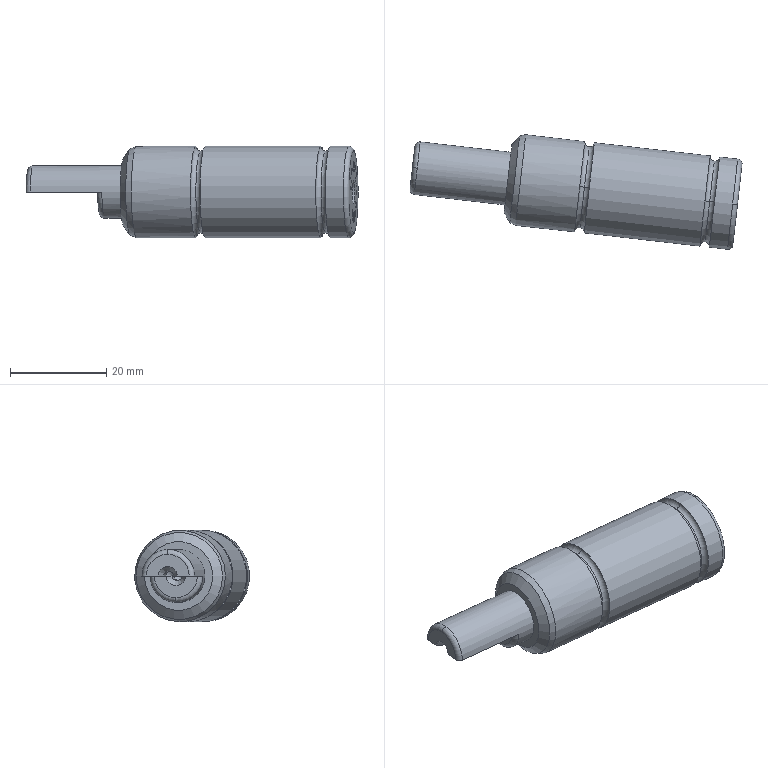Part | NX | features XQ 2 | 1 solid | 168 faces | box 69.047 x 23.908 x 19 mm | volume 14345 mm3 | plane 110 | spline 31 | torus 14 | cylinder 7 | cone 6 | commonest cylinder face diameters 19 x3 2 x2 4.9 x1 11 x1